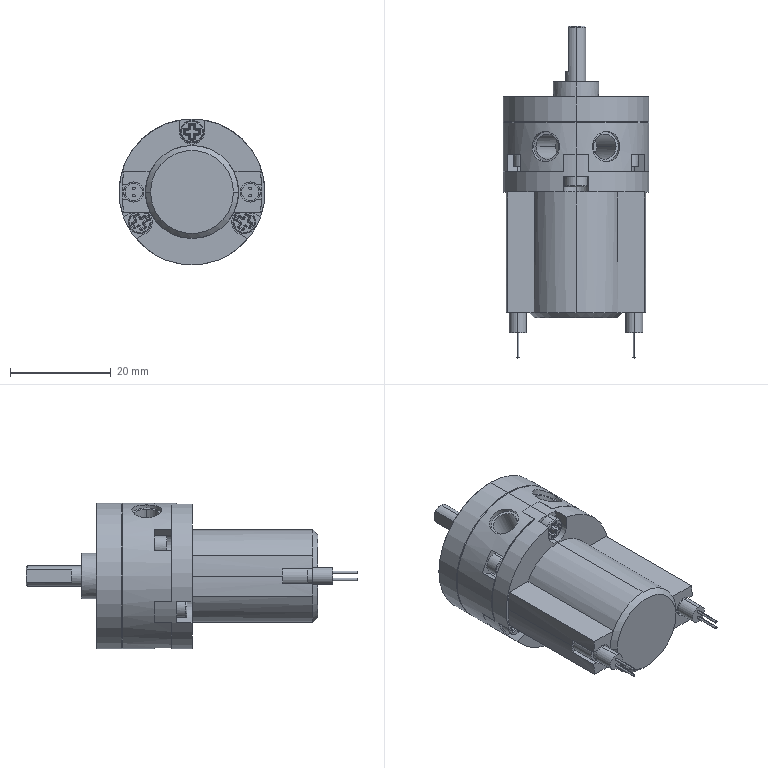Part | NX | 7 solids | 505 faces | box 29 x 66 x 29 mm | volume 20118 mm3 | cylinder 233 | plane 156 | torus 48 | sphere 36 | cone 32 | commonest cylinder face diameters 0.4 x114 4 x22 5 x21 3.4 x16 3 x14 0.5 x8